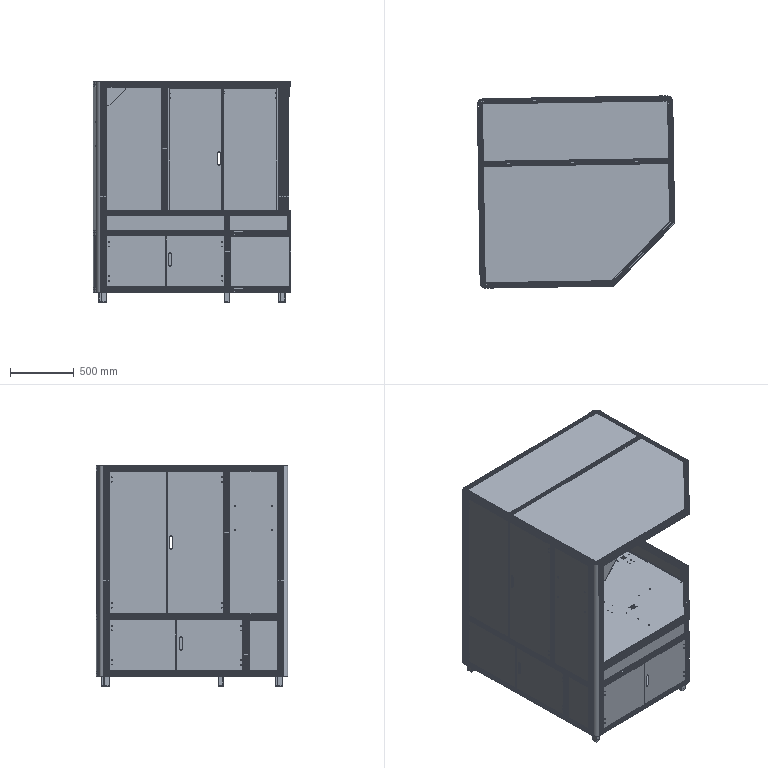Part | 91 solids | 6321 faces | volume 92285657 mm3 | plane 4345 | cylinder 1672 | spline 260 | torus 38 | sphere 6 | commonest cylinder face diameters 2 x230 6.8 x186 7 x144 1.473 x126 3.873 x118 5 x106